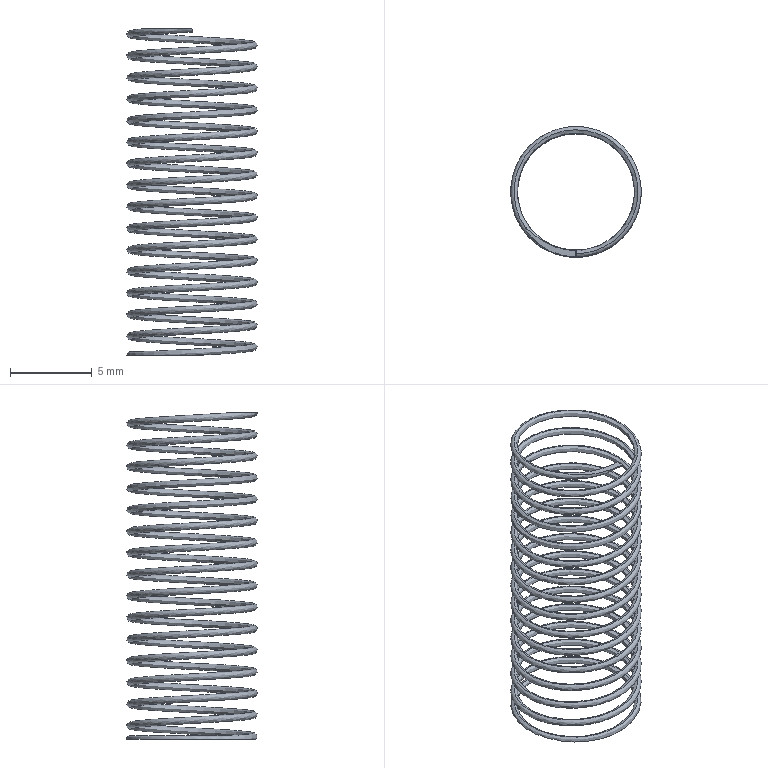Part | SolidWorks | features BaseBody 1 | 1 solid | 6 faces | box 8.007 x 8.002 x 20 mm | volume 45.848 mm3 | plane 4 | spline 2